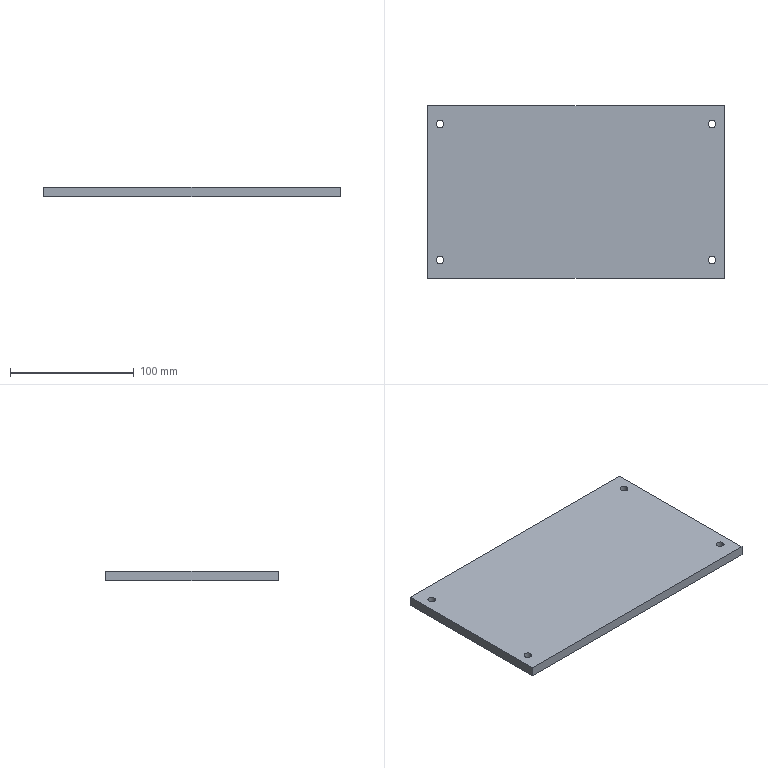Part | SolidWorks | features BaseBody 1 | 1 solid | 14 faces | box 240 x 140 x 8 mm | volume 267802 mm3 | cylinder 8 | plane 6 | commonest cylinder face diameters 6.3 x8
STEP:
#1=CARTESIAN_POINT('',(106.85,55.,-4.));
#2=VERTEX_POINT('',#1);
#3=CARTESIAN_POINT('',(113.15,55.,-4.));
#4=VERTEX_POINT('',#3);
#5=CARTESIAN_POINT('',(110.,55.,-4.));
#6=DIRECTION('',(0.,0.,1.));
#7=DIRECTION('',(1.,0.,0.));
#8=AXIS2_PLACEMENT_3D('',#5,#6,#7);
#9=CIRCLE('',#8,3.15);
#10=EDGE_CURVE('',#2,#4,#9,.T.);
#11=ORIENTED_EDGE('',*,*,#10,.F.);
#12=CARTESIAN_POINT('',(106.85,55.,4.));
#13=VERTEX_POINT('',#12);
#14=CARTESIAN_POINT('',(106.85,55.,-14.2));
#15=DIRECTION('',(0.,0.,1.));
#16=VECTOR('',#15,1000.);
#17=LINE('',#14,#16);
#18=EDGE_CURVE('',#2,#13,#17,.T.);
#19=ORIENTED_EDGE('',*,*,#18,.T.);
#20=CARTESIAN_POINT('',(113.15,55.,4.));
#21=VERTEX_POINT('',#20);
#22=CARTESIAN_POINT('',(110.,55.,4.));
#23=DIRECTION('',(0.,0.,-1.));
#24=DIRECTION('',(1.,0.,0.));
#25=AXIS2_PLACEMENT_3D('',#22,#23,#24);
#26=CIRCLE('',#25,3.15);
#27=EDGE_CURVE('',#21,#13,#26,.T.);
#28=ORIENTED_EDGE('',*,*,#27,.F.);
#29=CARTESIAN_POINT('',(113.15,55.,-14.2));
#30=DIRECTION('',(0.,0.,1.));
#31=VECTOR('',#30,1000.);
#32=LINE('',#29,#31);
#33=EDGE_CURVE('',#4,#21,#32,.T.);
#34=ORIENTED_EDGE('',*,*,#33,.F.);
#35=EDGE_LOOP('',(#11,#19,#28,#34));
#36=FACE_OUTER_BOUND('',#35,.T.);
#37=CARTESIAN_POINT('',(110.,55.,-14.2));
#38=DIRECTION('',(0.,0.,1.));
#39=DIRECTION('',(1.,0.,0.));
#40=AXIS2_PLACEMENT_3D('',#37,#38,#39);
#41=CYLINDRICAL_SURFACE('',#40,3.15);
#42=ADVANCED_FACE('',(#36),#41,.F.);
#43=CARTESIAN_POINT('',(-113.15,55.,-4.));
#44=VERTEX_POINT('',#43);
#45=CARTESIAN_POINT('',(-106.85,55.,-4.));
#46=VERTEX_POINT('',#45);
#47=CARTESIAN_POINT('',(-110.,55.,-4.));
#48=DIRECTION('',(0.,0.,1.));
#49=DIRECTION('',(1.,0.,0.));
#50=AXIS2_PLACEMENT_3D('',#47,#48,#49);
#51=CIRCLE('',#50,3.15);
#52=EDGE_CURVE('',#44,#46,#51,.T.);
#53=ORIENTED_EDGE('',*,*,#52,.F.);
#54=CARTESIAN_POINT('',(-113.15,55.,4.));
#55=VERTEX_POINT('',#54);
#56=CARTESIAN_POINT('',(-113.15,55.,-14.2));
#57=DIRECTION('',(0.,0.,1.));
#58=VECTOR('',#57,1000.);
#59=LINE('',#56,#58);
#60=EDGE_CURVE('',#44,#55,#59,.T.);
#61=ORIENTED_EDGE('',*,*,#60,.T.);
#62=CARTESIAN_POINT('',(-106.85,55.,4.));
#63=VERTEX_POINT('',#62);
#64=CARTESIAN_POINT('',(-110.,55.,4.));
#65=DIRECTION('',(0.,0.,-1.));
#66=DIRECTION('',(1.,0.,0.));
#67=AXIS2_PLACEMENT_3D('',#64,#65,#66);
#68=CIRCLE('',#67,3.15);
#69=EDGE_CURVE('',#63,#55,#68,.T.);
#70=ORIENTED_EDGE('',*,*,#69,.F.);
#71=CARTESIAN_POINT('',(-106.85,55.,-14.2));
#72=DIRECTION('',(0.,0.,1.));
#73=VECTOR('',#72,1000.);
#74=LINE('',#71,#73);
#75=EDGE_CURVE('',#46,#63,#74,.T.);
#76=ORIENTED_EDGE('',*,*,#75,.F.);
#77=EDGE_LOOP('',(#53,#61,#70,#76));
#78=FACE_OUTER_BOUND('',#77,.T.);
#79=CARTESIAN_POINT('',(-110.,55.,-14.2));
#80=DIRECTION('',(0.,0.,1.));
#81=DIRECTION('',(1.,0.,0.));
#82=AXIS2_PLACEMENT_3D('',#79,#80,#81);
#83=CYLINDRICAL_SURFACE('',#82,3.15);
#84=ADVANCED_FACE('',(#78),#83,.F.);
#85=CARTESIAN_POINT('',(106.85,-55.,-4.));
#86=VERTEX_POINT('',#85);
#87=CARTESIAN_POINT('',(113.15,-55.,-4.));
#88=VERTEX_POINT('',#87);
#89=CARTESIAN_POINT('',(110.,-55.,-4.));
#90=DIRECTION('',(0.,0.,1.));
#91=DIRECTION('',(1.,0.,0.));
#92=AXIS2_PLACEMENT_3D('',#89,#90,#91);
#93=CIRCLE('',#92,3.15);
#94=EDGE_CURVE('',#86,#88,#93,.T.);
#95=ORIENTED_EDGE('',*,*,#94,.F.);
#96=CARTESIAN_POINT('',(106.85,-55.,4.));
#97=VERTEX_POINT('',#96);
#98=CARTESIAN_POINT('',(106.85,-55.,-14.2));
#99=DIRECTION('',(0.,0.,1.));
#100=VECTOR('',#99,1000.);
#101=LINE('',#98,#100);
#102=EDGE_CURVE('',#86,#97,#101,.T.);
#103=ORIENTED_EDGE('',*,*,#102,.T.);
#104=CARTESIAN_POINT('',(113.15,-55.,4.));
#105=VERTEX_POINT('',#104);
#106=CARTESIAN_POINT('',(110.,-55.,4.));
#107=DIRECTION('',(0.,0.,-1.));
#108=DIRECTION('',(1.,0.,0.));
#109=AXIS2_PLACEMENT_3D('',#106,#107,#108);
#110=CIRCLE('',#109,3.15);
#111=EDGE_CURVE('',#105,#97,#110,.T.);
#112=ORIENTED_EDGE('',*,*,#111,.F.);
#113=CARTESIAN_POINT('',(113.15,-55.,-14.2));
#114=DIRECTION('',(0.,0.,1.));
#115=VECTOR('',#114,1000.);
#116=LINE('',#113,#115);
#117=EDGE_CURVE('',#88,#105,#116,.T.);
#118=ORIENTED_EDGE('',*,*,#117,.F.);
#119=EDGE_LOOP('',(#95,#103,#112,#118));
#120=FACE_OUTER_BOUND('',#119,.T.);
#121=CARTESIAN_POINT('',(110.,-55.,-14.2));
#122=DIRECTION('',(0.,0.,1.));
#123=DIRECTION('',(1.,0.,0.));
#124=AXIS2_PLACEMENT_3D('',#121,#122,#123);
#125=CYLINDRICAL_SURFACE('',#124,3.15);
#126=ADVANCED_FACE('',(#120),#125,.F.);
#127=CARTESIAN_POINT('',(-113.15,-55.,-4.));
#128=VERTEX_POINT('',#127);
#129=CARTESIAN_POINT('',(-106.85,-55.,-4.));
#130=VERTEX_POINT('',#129);
#131=CARTESIAN_POINT('',(-110.,-55.,-4.));
#132=DIRECTION('',(0.,0.,1.));
#133=DIRECTION('',(1.,0.,0.));
#134=AXIS2_PLACEMENT_3D('',#131,#132,#133);
#135=CIRCLE('',#134,3.15);
#136=EDGE_CURVE('',#128,#130,#135,.T.);
#137=ORIENTED_EDGE('',*,*,#136,.F.);
#138=CARTESIAN_POINT('',(-113.15,-55.,4.));
#139=VERTEX_POINT('',#138);
#140=CARTESIAN_POINT('',(-113.15,-55.,-14.2));
#141=DIRECTION('',(0.,0.,1.));
#142=VECTOR('',#141,1000.);
#143=LINE('',#140,#142);
#144=EDGE_CURVE('',#128,#139,#143,.T.);
#145=ORIENTED_EDGE('',*,*,#144,.T.);
#146=CARTESIAN_POINT('',(-106.85,-55.,4.));
#147=VERTEX_POINT('',#146);
#148=CARTESIAN_POINT('',(-110.,-55.,4.));
#149=DIRECTION('',(0.,0.,-1.));
#150=DIRECTION('',(1.,0.,0.));
#151=AXIS2_PLACEMENT_3D('',#148,#149,#150);
#152=CIRCLE('',#151,3.15);
#153=EDGE_CURVE('',#147,#139,#152,.T.);
#154=ORIENTED_EDGE('',*,*,#153,.F.);
#155=CARTESIAN_POINT('',(-106.85,-55.,-14.2));
#156=DIRECTION('',(0.,0.,1.));
#157=VECTOR('',#156,1000.);
#158=LINE('',#155,#157);
#159=EDGE_CURVE('',#130,#147,#158,.T.);
#160=ORIENTED_EDGE('',*,*,#159,.F.);
#161=EDGE_LOOP('',(#137,#145,#154,#160));
#162=FACE_OUTER_BOUND('',#161,.T.);
#163=CARTESIAN_POINT('',(-110.,-55.,-14.2));
#164=DIRECTION('',(0.,0.,1.));
#165=DIRECTION('',(1.,0.,0.));
#166=AXIS2_PLACEMENT_3D('',#163,#164,#165);
#167=CYLINDRICAL_SURFACE('',#166,3.15);
#168=ADVANCED_FACE('',(#162),#167,.F.);
#169=ORIENTED_EDGE('',*,*,#27,.T.);
#170=CARTESIAN_POINT('',(110.,55.,4.));
#171=DIRECTION('',(0.,0.,-1.));
#172=DIRECTION('',(1.,0.,0.));
#173=AXIS2_PLACEMENT_3D('',#170,#171,#172);
#174=CIRCLE('',#173,3.15);
#175=EDGE_CURVE('',#13,#21,#174,.T.);
#176=ORIENTED_EDGE('',*,*,#175,.T.);
#177=EDGE_LOOP('',(#169,#176));
#178=FACE_BOUND('',#177,.T.);
#179=ORIENTED_EDGE('',*,*,#69,.T.);
#180=CARTESIAN_POINT('',(-110.,55.,4.));
#181=DIRECTION('',(0.,0.,-1.));
#182=DIRECTION('',(1.,0.,0.));
#183=AXIS2_PLACEMENT_3D('',#180,#181,#182);
#184=CIRCLE('',#183,3.15);
#185=EDGE_CURVE('',#55,#63,#184,.T.);
#186=ORIENTED_EDGE('',*,*,#185,.T.);
#187=EDGE_LOOP('',(#179,#186));
#188=FACE_BOUND('',#187,.T.);
#189=ORIENTED_EDGE('',*,*,#111,.T.);
#190=CARTESIAN_POINT('',(110.,-55.,4.));
#191=DIRECTION('',(0.,0.,-1.));
#192=DIRECTION('',(1.,0.,0.));
#193=AXIS2_PLACEMENT_3D('',#190,#191,#192);
#194=CIRCLE('',#193,3.15);
#195=EDGE_CURVE('',#97,#105,#194,.T.);
#196=ORIENTED_EDGE('',*,*,#195,.T.);
#197=EDGE_LOOP('',(#189,#196));
#198=FACE_BOUND('',#197,.T.);
#199=ORIENTED_EDGE('',*,*,#153,.T.);
#200=CARTESIAN_POINT('',(-110.,-55.,4.));
#201=DIRECTION('',(0.,0.,-1.));
#202=DIRECTION('',(1.,0.,0.));
#203=AXIS2_PLACEMENT_3D('',#200,#201,#202);
#204=CIRCLE('',#203,3.15);
#205=EDGE_CURVE('',#139,#147,#204,.T.);
#206=ORIENTED_EDGE('',*,*,#205,.T.);
#207=EDGE_LOOP('',(#199,#206));
#208=FACE_BOUND('',#207,.T.);
#209=CARTESIAN_POINT('',(120.,-70.,4.));
#210=VERTEX_POINT('',#209);
#211=CARTESIAN_POINT('',(120.,70.,4.));
#212=VERTEX_POINT('',#211);
#213=CARTESIAN_POINT('',(120.,-70.,4.));
#214=DIRECTION('',(0.,1.,0.));
#215=VECTOR('',#214,1000.);
#216=LINE('',#213,#215);
#217=EDGE_CURVE('',#210,#212,#216,.T.);
#218=ORIENTED_EDGE('',*,*,#217,.T.);
#219=CARTESIAN_POINT('',(-120.,70.,4.));
#220=VERTEX_POINT('',#219);
#221=CARTESIAN_POINT('',(-120.,70.,4.));
#222=DIRECTION('',(-1.,0.,0.));
#223=VECTOR('',#222,1000.);
#224=LINE('',#221,#223);
#225=EDGE_CURVE('',#212,#220,#224,.T.);
#226=ORIENTED_EDGE('',*,*,#225,.T.);
#227=CARTESIAN_POINT('',(-120.,-70.,4.));
#228=VERTEX_POINT('',#227);
#229=CARTESIAN_POINT('',(-120.,-70.,4.));
#230=DIRECTION('',(0.,-1.,0.));
#231=VECTOR('',#230,1000.);
#232=LINE('',#229,#231);
#233=EDGE_CURVE('',#220,#228,#232,.T.);
#234=ORIENTED_EDGE('',*,*,#233,.T.);
#235=CARTESIAN_POINT('',(-120.,-70.,4.));
#236=DIRECTION('',(1.,0.,0.));
#237=VECTOR('',#236,1000.);
#238=LINE('',#235,#237);
#239=EDGE_CURVE('',#228,#210,#238,.T.);
#240=ORIENTED_EDGE('',*,*,#239,.T.);
#241=EDGE_LOOP('',(#218,#226,#234,#240));
#242=FACE_OUTER_BOUND('',#241,.T.);
#243=CARTESIAN_POINT('',(-120.,-70.,4.));
#244=DIRECTION('',(0.,0.,1.));
#245=DIRECTION('',(1.,0.,0.));
#246=AXIS2_PLACEMENT_3D('',#243,#244,#245);
#247=PLANE('',#246);
#248=ADVANCED_FACE('',(#178,#188,#198,#208,#242),#247,.T.);
#249=ORIENTED_EDGE('',*,*,#18,.F.);
#250=CARTESIAN_POINT('',(110.,55.,-4.));
#251=DIRECTION('',(0.,0.,1.));
#252=DIRECTION('',(1.,0.,0.));
#253=AXIS2_PLACEMENT_3D('',#250,#251,#252);
#254=CIRCLE('',#253,3.15);
#255=EDGE_CURVE('',#4,#2,#254,.T.);
#256=ORIENTED_EDGE('',*,*,#255,.F.);
#257=ORIENTED_EDGE('',*,*,#33,.T.);
#258=ORIENTED_EDGE('',*,*,#175,.F.);
#259=EDGE_LOOP('',(#249,#256,#257,#258));
#260=FACE_OUTER_BOUND('',#259,.T.);
#261=CARTESIAN_POINT('',(110.,55.,-14.2));
#262=DIRECTION('',(0.,0.,1.));
#263=DIRECTION('',(1.,0.,0.));
#264=AXIS2_PLACEMENT_3D('',#261,#262,#263);
#265=CYLINDRICAL_SURFACE('',#264,3.15);
#266=ADVANCED_FACE('',(#260),#265,.F.);
#267=ORIENTED_EDGE('',*,*,#60,.F.);
#268=CARTESIAN_POINT('',(-110.,55.,-4.));
#269=DIRECTION('',(0.,0.,1.));
#270=DIRECTION('',(1.,0.,0.));
#271=AXIS2_PLACEMENT_3D('',#268,#269,#270);
#272=CIRCLE('',#271,3.15);
#273=EDGE_CURVE('',#46,#44,#272,.T.);
#274=ORIENTED_EDGE('',*,*,#273,.F.);
#275=ORIENTED_EDGE('',*,*,#75,.T.);
#276=ORIENTED_EDGE('',*,*,#185,.F.);
#277=EDGE_LOOP('',(#267,#274,#275,#276));
#278=FACE_OUTER_BOUND('',#277,.T.);
#279=CARTESIAN_POINT('',(-110.,55.,-14.2));
#280=DIRECTION('',(0.,0.,1.));
#281=DIRECTION('',(1.,0.,0.));
#282=AXIS2_PLACEMENT_3D('',#279,#280,#281);
#283=CYLINDRICAL_SURFACE('',#282,3.15);
#284=ADVANCED_FACE('',(#278),#283,.F.);
#285=ORIENTED_EDGE('',*,*,#102,.F.);
#286=CARTESIAN_POINT('',(110.,-55.,-4.));
#287=DIRECTION('',(0.,0.,1.));
#288=DIRECTION('',(1.,0.,0.));
#289=AXIS2_PLACEMENT_3D('',#286,#287,#288);
#290=CIRCLE('',#289,3.15);
#291=EDGE_CURVE('',#88,#86,#290,.T.);
#292=ORIENTED_EDGE('',*,*,#291,.F.);
#293=ORIENTED_EDGE('',*,*,#117,.T.);
#294=ORIENTED_EDGE('',*,*,#195,.F.);
#295=EDGE_LOOP('',(#285,#292,#293,#294));
#296=FACE_OUTER_BOUND('',#295,.T.);
#297=CARTESIAN_POINT('',(110.,-55.,-14.2));
#298=DIRECTION('',(0.,0.,1.));
#299=DIRECTION('',(1.,0.,0.));
#300=AXIS2_PLACEMENT_3D('',#297,#298,#299);
#301=CYLINDRICAL_SURFACE('',#300,3.15);
#302=ADVANCED_FACE('',(#296),#301,.F.);
#303=ORIENTED_EDGE('',*,*,#144,.F.);
#304=CARTESIAN_POINT('',(-110.,-55.,-4.));
#305=DIRECTION('',(0.,0.,1.));
#306=DIRECTION('',(1.,0.,0.));
#307=AXIS2_PLACEMENT_3D('',#304,#305,#306);
#308=CIRCLE('',#307,3.15);
#309=EDGE_CURVE('',#130,#128,#308,.T.);
#310=ORIENTED_EDGE('',*,*,#309,.F.);
#311=ORIENTED_EDGE('',*,*,#159,.T.);
#312=ORIENTED_EDGE('',*,*,#205,.F.);
#313=EDGE_LOOP('',(#303,#310,#311,#312));
#314=FACE_OUTER_BOUND('',#313,.T.);
#315=CARTESIAN_POINT('',(-110.,-55.,-14.2));
#316=DIRECTION('',(0.,0.,1.));
#317=DIRECTION('',(1.,0.,0.));
#318=AXIS2_PLACEMENT_3D('',#315,#316,#317);
#319=CYLINDRICAL_SURFACE('',#318,3.15);
#320=ADVANCED_FACE('',(#314),#319,.F.);
#321=ORIENTED_EDGE('',*,*,#225,.F.);
#322=CARTESIAN_POINT('',(120.,70.,-4.));
#323=VERTEX_POINT('',#322);
#324=CARTESIAN_POINT('',(120.,70.,-4.));
#325=DIRECTION('',(0.,0.,-1.));
#326=VECTOR('',#325,1000.);
#327=LINE('',#324,#326);
#328=EDGE_CURVE('',#212,#323,#327,.T.);
#329=ORIENTED_EDGE('',*,*,#328,.T.);
#330=CARTESIAN_POINT('',(-120.,70.,-4.));
#331=VERTEX_POINT('',#330);
#332=CARTESIAN_POINT('',(-120.,70.,-4.));
#333=DIRECTION('',(-1.,0.,0.));
#334=VECTOR('',#333,1000.);
#335=LINE('',#332,#334);
#336=EDGE_CURVE('',#323,#331,#335,.T.);
#337=ORIENTED_EDGE('',*,*,#336,.T.);
#338=CARTESIAN_POINT('',(-120.,70.,-4.));
#339=DIRECTION('',(0.,0.,1.));
#340=VECTOR('',#339,1000.);
#341=LINE('',#338,#340);
#342=EDGE_CURVE('',#331,#220,#341,.T.);
#343=ORIENTED_EDGE('',*,*,#342,.T.);
#344=EDGE_LOOP('',(#321,#329,#337,#343));
#345=FACE_OUTER_BOUND('',#344,.T.);
#346=CARTESIAN_POINT('',(-120.,70.,-4.));
#347=DIRECTION('',(0.,1.,0.));
#348=DIRECTION('',(0.,0.,1.));
#349=AXIS2_PLACEMENT_3D('',#346,#347,#348);
#350=PLANE('',#349);
#351=ADVANCED_FACE('',(#345),#350,.T.);
#352=ORIENTED_EDGE('',*,*,#328,.F.);
#353=ORIENTED_EDGE('',*,*,#217,.F.);
#354=CARTESIAN_POINT('',(120.,-70.,-4.));
#355=VERTEX_POINT('',#354);
#356=CARTESIAN_POINT('',(120.,-70.,-4.));
#357=DIRECTION('',(0.,0.,-1.));
#358=VECTOR('',#357,1000.);
#359=LINE('',#356,#358);
#360=EDGE_CURVE('',#210,#355,#359,.T.);
#361=ORIENTED_EDGE('',*,*,#360,.T.);
#362=CARTESIAN_POINT('',(120.,-70.,-4.));
#363=DIRECTION('',(0.,1.,0.));
#364=VECTOR('',#363,1000.);
#365=LINE('',#362,#364);
#366=EDGE_CURVE('',#355,#323,#365,.T.);
#367=ORIENTED_EDGE('',*,*,#366,.T.);
#368=EDGE_LOOP('',(#352,#353,#361,#367));
#369=FACE_OUTER_BOUND('',#368,.T.);
#370=CARTESIAN_POINT('',(120.,-70.,-4.));
#371=DIRECTION('',(1.,0.,0.));
#372=DIRECTION('',(0.,0.,-1.));
#373=AXIS2_PLACEMENT_3D('',#370,#371,#372);
#374=PLANE('',#373);
#375=ADVANCED_FACE('',(#369),#374,.T.);
#376=ORIENTED_EDGE('',*,*,#239,.F.);
#377=CARTESIAN_POINT('',(-120.,-70.,-4.));
#378=VERTEX_POINT('',#377);
#379=CARTESIAN_POINT('',(-120.,-70.,-4.));
#380=DIRECTION('',(0.,0.,1.));
#381=VECTOR('',#380,1000.);
#382=LINE('',#379,#381);
#383=EDGE_CURVE('',#378,#228,#382,.T.);
#384=ORIENTED_EDGE('',*,*,#383,.F.);
#385=CARTESIAN_POINT('',(-120.,-70.,-4.));
#386=DIRECTION('',(-1.,0.,0.));
#387=VECTOR('',#386,1000.);
#388=LINE('',#385,#387);
#389=EDGE_CURVE('',#355,#378,#388,.T.);
#390=ORIENTED_EDGE('',*,*,#389,.F.);
#391=ORIENTED_EDGE('',*,*,#360,.F.);
#392=EDGE_LOOP('',(#376,#384,#390,#391));
#393=FACE_OUTER_BOUND('',#392,.T.);
#394=CARTESIAN_POINT('',(-120.,-70.,-4.));
#395=DIRECTION('',(0.,1.,0.));
#396=DIRECTION('',(0.,0.,1.));
#397=AXIS2_PLACEMENT_3D('',#394,#395,#396);
#398=PLANE('',#397);
#399=ADVANCED_FACE('',(#393),#398,.F.);
#400=ORIENTED_EDGE('',*,*,#342,.F.);
#401=CARTESIAN_POINT('',(-120.,-70.,-4.));
#402=DIRECTION('',(0.,1.,0.));
#403=VECTOR('',#402,1000.);
#404=LINE('',#401,#403);
#405=EDGE_CURVE('',#378,#331,#404,.T.);
#406=ORIENTED_EDGE('',*,*,#405,.F.);
#407=ORIENTED_EDGE('',*,*,#383,.T.);
#408=ORIENTED_EDGE('',*,*,#233,.F.);
#409=EDGE_LOOP('',(#400,#406,#407,#408));
#410=FACE_OUTER_BOUND('',#409,.T.);
#411=CARTESIAN_POINT('',(-120.,-70.,-4.));
#412=DIRECTION('',(1.,0.,0.));
#413=DIRECTION('',(0.,0.,-1.));
#414=AXIS2_PLACEMENT_3D('',#411,#412,#413);
#415=PLANE('',#414);
#416=ADVANCED_FACE('',(#410),#415,.F.);
#417=ORIENTED_EDGE('',*,*,#255,.T.);
#418=ORIENTED_EDGE('',*,*,#10,.T.);
#419=EDGE_LOOP('',(#417,#418));
#420=FACE_BOUND('',#419,.T.);
#421=ORIENTED_EDGE('',*,*,#273,.T.);
#422=ORIENTED_EDGE('',*,*,#52,.T.);
#423=EDGE_LOOP('',(#421,#422));
#424=FACE_BOUND('',#423,.T.);
#425=ORIENTED_EDGE('',*,*,#291,.T.);
#426=ORIENTED_EDGE('',*,*,#94,.T.);
#427=EDGE_LOOP('',(#425,#426));
#428=FACE_BOUND('',#427,.T.);
#429=ORIENTED_EDGE('',*,*,#309,.T.);
#430=ORIENTED_EDGE('',*,*,#136,.T.);
#431=EDGE_LOOP('',(#429,#430));
#432=FACE_BOUND('',#431,.T.);
#433=ORIENTED_EDGE('',*,*,#366,.F.);
#434=ORIENTED_EDGE('',*,*,#389,.T.);
#435=ORIENTED_EDGE('',*,*,#405,.T.);
#436=ORIENTED_EDGE('',*,*,#336,.F.);
#437=EDGE_LOOP('',(#433,#434,#435,#436));
#438=FACE_OUTER_BOUND('',#437,.T.);
#439=CARTESIAN_POINT('',(-120.,-70.,-4.));
#440=DIRECTION('',(0.,0.,1.));
#441=DIRECTION('',(1.,0.,0.));
#442=AXIS2_PLACEMENT_3D('',#439,#440,#441);
#443=PLANE('',#442);
#444=ADVANCED_FACE('',(#420,#424,#428,#432,#438),#443,.F.);
#445=CLOSED_SHELL('',(#42,#84,#126,#168,#248,#266,#284,#302,#320,#351,#375,#399,#416,#444));
#446=MANIFOLD_SOLID_BREP('',#445);
#447=CARTESIAN_POINT('',(0.,0.,0.));
#448=DIRECTION('',(0.,0.,1.));
#449=DIRECTION('',(1.,0.,0.));
#450=AXIS2_PLACEMENT_3D('',#447,#448,#449);
#451=(LENGTH_UNIT()NAMED_UNIT(*)SI_UNIT(.MILLI.,.METRE.));
#452=UNCERTAINTY_MEASURE_WITH_UNIT(LENGTH_MEASURE(0.00001),#451,'','');
#453=(NAMED_UNIT(*)PLANE_ANGLE_UNIT()SI_UNIT($,.RADIAN.));
#454=(NAMED_UNIT(*)SI_UNIT($,.STERADIAN.)SOLID_ANGLE_UNIT());
#455=(GEOMETRIC_REPRESENTATION_CONTEXT(3)GLOBAL_UNCERTAINTY_ASSIGNED_CONTEXT((#452))GLOBAL_UNIT_ASSIGNED_CONTEXT((#451,#453,#454))REPRESENTATION_CONTEXT('',''));
#456=ADVANCED_BREP_SHAPE_REPRESENTATION('',(#446,#450),#455);